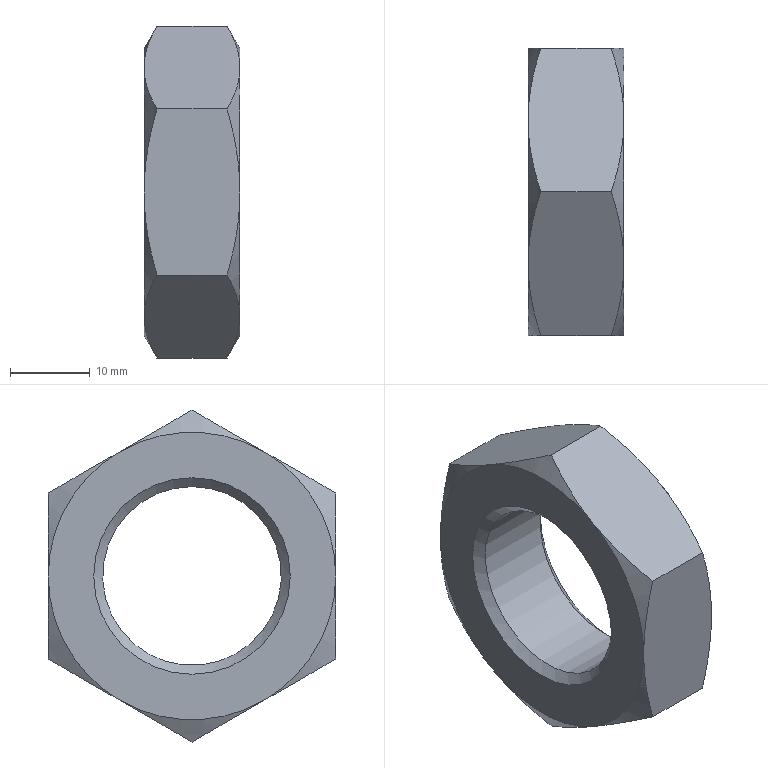Part | STEP file | Tube necking machine_id622_x_t | 1 solid | 23 faces | box 12 x 36 x 41.569 mm | volume 8555 mm3 | cone 14 | plane 8 | cylinder 1 | commonest cylinder face diameters 22.376 x1